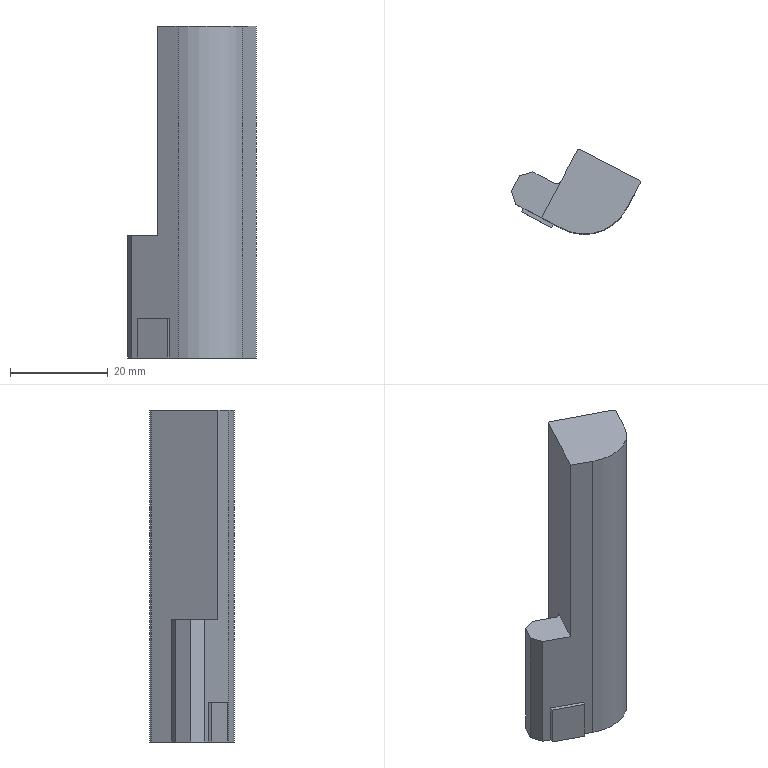Part | STEP file | gslz 2016.10.28-13_id278_x_t | 1 solid | 19 faces | box 26.348 x 17.329 x 68 mm | volume 15925 mm3 | plane 14 | cylinder 4 | other 1 | commonest cylinder face diameters 1 x2 2 x1 19.5 x1